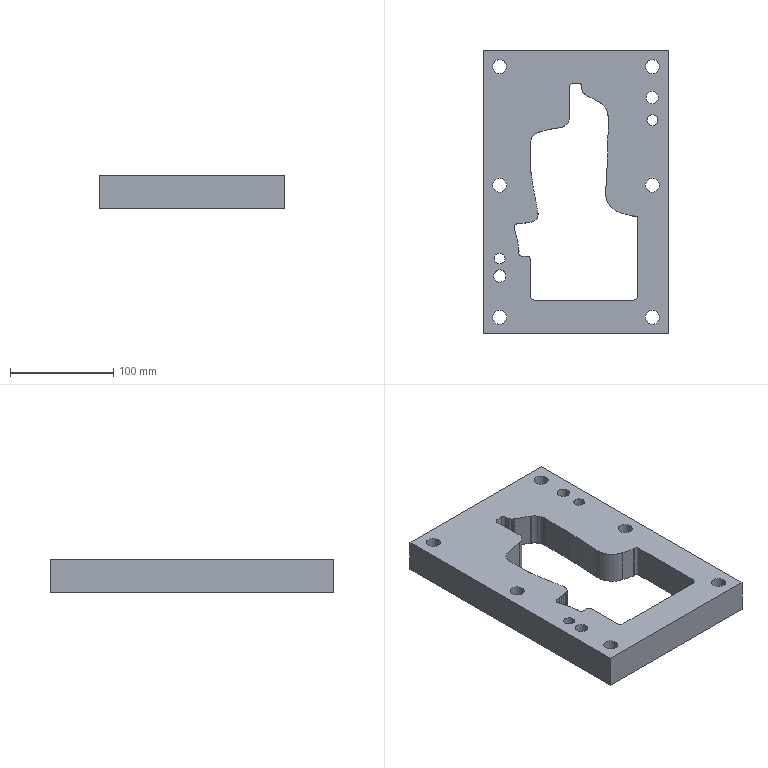Part | STEP file | lll_id3198_x_t | 1 solid | 101 faces | box 180 x 275 x 32 mm | volume 1007156 mm3 | cylinder 80 | plane 21 | commonest cylinder face diameters 6 x7 13.509 x6 20.008 x6 10 x2 10.505 x2 12 x2